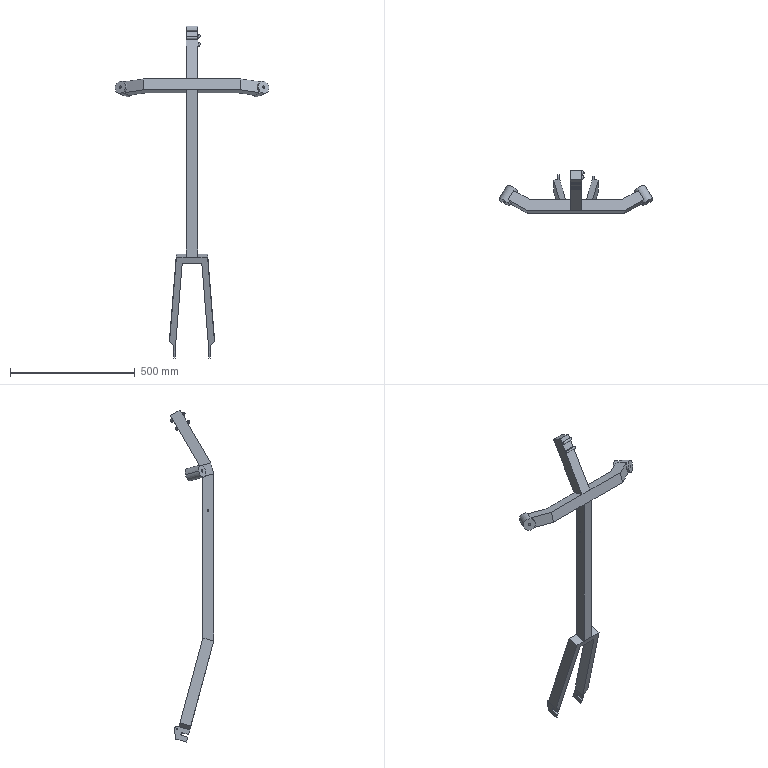Part | STEP file | Cobra Frame | 1 solid | 91 faces | box 616.506 x 173.118 x 1330 mm | volume 4060018 mm3 | plane 61 | cylinder 30 | commonest cylinder face diameters 10 x8 6.5 x4 11 x4 15 x4 50 x4 5.1 x2